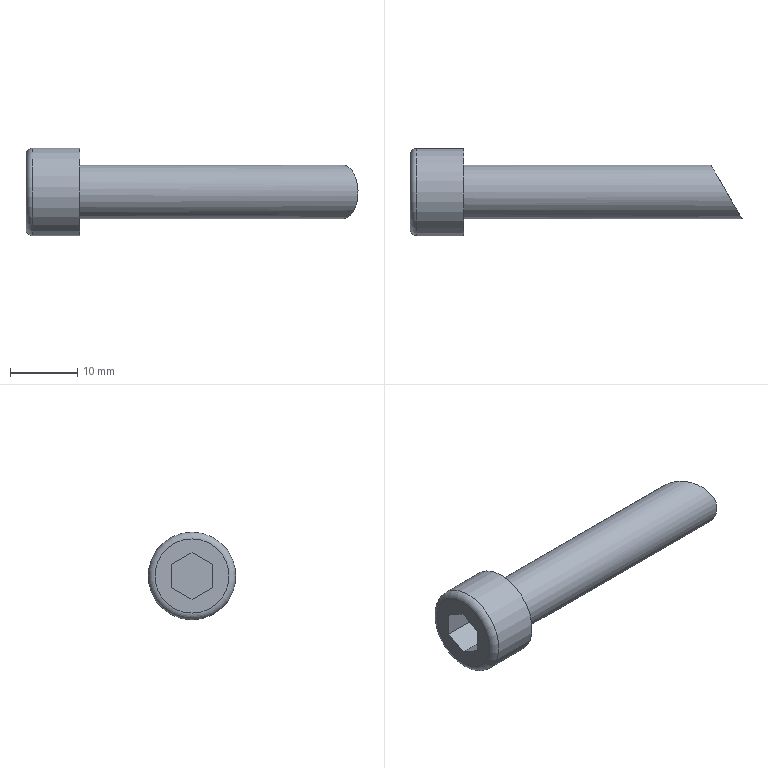Part | STEP file | Tube necking machine_id610_x_t | 1 solid | 13 faces | box 49.238 x 13 x 13 mm | volume 2846 mm3 | plane 10 | cylinder 2 | torus 1 | commonest cylinder face diameters 8 x1 13 x1
STEP:
#1=CARTESIAN_POINT('',(0.,0.,0.));
#2=DIRECTION('',(0.,0.,1.));
#3=DIRECTION('',(1.,0.,0.));
#4=AXIS2_PLACEMENT_3D('',#1,#2,#3);
#5=CARTESIAN_POINT('',(367.5,30.,164.5));
#6=VERTEX_POINT('',#5);
#7=CARTESIAN_POINT('',(367.5,30.,170.));
#8=DIRECTION('',(-1.,0.,0.));
#9=DIRECTION('',(0.,0.,-1.));
#10=AXIS2_PLACEMENT_3D('',#7,#8,#9);
#11=CIRCLE('',#10,5.5);
#12=CARTESIAN_POINT('',(367.5,30.,176.5));
#13=DIRECTION('',(1.,0.,0.));
#14=DIRECTION('',(0.,0.,-1.));
#15=AXIS2_PLACEMENT_3D('',#12,#13,#14);
#16=PLANE('',#15);
#17=CARTESIAN_POINT('',(12.,0.));
#18=CARTESIAN_POINT('',(12.,-9.526));
#19=CARTESIAN_POINT('',(3.75,-4.763));
#20=CARTESIAN_POINT('',(-4.5,0.));
#21=CARTESIAN_POINT('',(3.75,4.763));
#22=CARTESIAN_POINT('',(12.,9.526));
#23=CARTESIAN_POINT('',(12.,0.));
#24=(BOUNDED_CURVE()B_SPLINE_CURVE(2,(#17,#18,#19,#20,#21,#22,#23),.UNSPECIFIED.,.T.,.F.)B_SPLINE_CURVE_WITH_KNOTS((1,2,2,2,2,1),(-2.094,0.,2.094,4.189,6.283,8.378),.UNSPECIFIED.)CURVE()GEOMETRIC_REPRESENTATION_ITEM()RATIONAL_B_SPLINE_CURVE((1.,0.5,1.,0.5,1.,0.5,1.))REPRESENTATION_ITEM(''));
#25=(GEOMETRIC_REPRESENTATION_CONTEXT(2)PARAMETRIC_REPRESENTATION_CONTEXT()REPRESENTATION_CONTEXT('',''));
#26=DEFINITIONAL_REPRESENTATION('',(#24),#25);
#27=PCURVE('',#16,#26);
#28=CARTESIAN_POINT('',(368.5,30.,170.));
#29=DIRECTION('',(1.,0.,0.));
#30=DIRECTION('',(0.,0.,-1.));
#31=AXIS2_PLACEMENT_3D('',#28,#29,#30);
#32=TOROIDAL_SURFACE('',#31,5.5,1.);
#33=CARTESIAN_POINT('',(6.283,4.712));
#34=DIRECTION('',(-1.,0.));
#35=VECTOR('',#34,1.);
#36=LINE('',#33,#35);
#37=(GEOMETRIC_REPRESENTATION_CONTEXT(2)PARAMETRIC_REPRESENTATION_CONTEXT()REPRESENTATION_CONTEXT('',''));
#38=DEFINITIONAL_REPRESENTATION('',(#36),#37);
#39=PCURVE('',#32,#38);
#40=SURFACE_CURVE('',#11,(#27,#39),.PCURVE_S1.);
#41=EDGE_CURVE('',#6,#6,#40,.T.);
#42=ORIENTED_EDGE('',*,*,#41,.T.);
#43=EDGE_LOOP('',(#42));
#44=FACE_BOUND('',#43,.T.);
#45=CARTESIAN_POINT('',(367.5,33.,168.268));
#46=VERTEX_POINT('',#45);
#47=CARTESIAN_POINT('',(367.5,33.,171.732));
#48=VERTEX_POINT('',#47);
#49=CARTESIAN_POINT('',(367.5,33.,168.268));
#50=DIRECTION('',(0.,0.,1.));
#51=VECTOR('',#50,1.);
#52=LINE('',#49,#51);
#53=CARTESIAN_POINT('',(8.232,3.));
#54=DIRECTION('',(-1.,0.));
#55=VECTOR('',#54,1.);
#56=LINE('',#53,#55);
#57=(GEOMETRIC_REPRESENTATION_CONTEXT(2)PARAMETRIC_REPRESENTATION_CONTEXT()REPRESENTATION_CONTEXT('',''));
#58=DEFINITIONAL_REPRESENTATION('',(#56),#57);
#59=PCURVE('',#16,#58);
#60=CARTESIAN_POINT('',(372.78,33.,168.268));
#61=DIRECTION('',(0.,-1.,0.));
#62=DIRECTION('',(0.,0.,1.));
#63=AXIS2_PLACEMENT_3D('',#60,#61,#62);
#64=PLANE('',#63);
#65=CARTESIAN_POINT('',(0.,5.28));
#66=DIRECTION('',(1.,0.));
#67=VECTOR('',#66,1.);
#68=LINE('',#65,#67);
#69=(GEOMETRIC_REPRESENTATION_CONTEXT(2)PARAMETRIC_REPRESENTATION_CONTEXT()REPRESENTATION_CONTEXT('',''));
#70=DEFINITIONAL_REPRESENTATION('',(#68),#69);
#71=PCURVE('',#64,#70);
#72=SURFACE_CURVE('',#52,(#59,#71),.PCURVE_S1.);
#73=EDGE_CURVE('',#46,#48,#72,.T.);
#74=ORIENTED_EDGE('',*,*,#73,.T.);
#75=CARTESIAN_POINT('',(367.5,30.,173.464));
#76=VERTEX_POINT('',#75);
#77=CARTESIAN_POINT('',(367.5,33.,171.732));
#78=DIRECTION('',(0.,-0.866,0.5));
#79=VECTOR('',#78,1.);
#80=LINE('',#77,#79);
#81=CARTESIAN_POINT('',(4.768,3.));
#82=DIRECTION('',(-0.5,-0.866));
#83=VECTOR('',#82,1.);
#84=LINE('',#81,#83);
#85=(GEOMETRIC_REPRESENTATION_CONTEXT(2)PARAMETRIC_REPRESENTATION_CONTEXT()REPRESENTATION_CONTEXT('',''));
#86=DEFINITIONAL_REPRESENTATION('',(#84),#85);
#87=PCURVE('',#16,#86);
#88=CARTESIAN_POINT('',(372.78,33.,171.732));
#89=DIRECTION('',(0.,-0.5,-0.866));
#90=DIRECTION('',(0.,-0.866,0.5));
#91=AXIS2_PLACEMENT_3D('',#88,#89,#90);
#92=PLANE('',#91);
#93=CARTESIAN_POINT('',(0.,5.28));
#94=DIRECTION('',(1.,0.));
#95=VECTOR('',#94,1.);
#96=LINE('',#93,#95);
#97=(GEOMETRIC_REPRESENTATION_CONTEXT(2)PARAMETRIC_REPRESENTATION_CONTEXT()REPRESENTATION_CONTEXT('',''));
#98=DEFINITIONAL_REPRESENTATION('',(#96),#97);
#99=PCURVE('',#92,#98);
#100=SURFACE_CURVE('',#80,(#87,#99),.PCURVE_S1.);
#101=EDGE_CURVE('',#48,#76,#100,.T.);
#102=ORIENTED_EDGE('',*,*,#101,.T.);
#103=CARTESIAN_POINT('',(367.5,27.,171.732));
#104=VERTEX_POINT('',#103);
#105=CARTESIAN_POINT('',(367.5,30.,173.464));
#106=DIRECTION('',(0.,-0.866,-0.5));
#107=VECTOR('',#106,1.);
#108=LINE('',#105,#107);
#109=CARTESIAN_POINT('',(3.036,0.));
#110=DIRECTION('',(0.5,-0.866));
#111=VECTOR('',#110,1.);
#112=LINE('',#109,#111);
#113=(GEOMETRIC_REPRESENTATION_CONTEXT(2)PARAMETRIC_REPRESENTATION_CONTEXT()REPRESENTATION_CONTEXT('',''));
#114=DEFINITIONAL_REPRESENTATION('',(#112),#113);
#115=PCURVE('',#16,#114);
#116=CARTESIAN_POINT('',(372.78,30.,173.464));
#117=DIRECTION('',(0.,0.5,-0.866));
#118=DIRECTION('',(0.,-0.866,-0.5));
#119=AXIS2_PLACEMENT_3D('',#116,#117,#118);
#120=PLANE('',#119);
#121=CARTESIAN_POINT('',(0.,5.28));
#122=DIRECTION('',(1.,0.));
#123=VECTOR('',#122,1.);
#124=LINE('',#121,#123);
#125=(GEOMETRIC_REPRESENTATION_CONTEXT(2)PARAMETRIC_REPRESENTATION_CONTEXT()REPRESENTATION_CONTEXT('',''));
#126=DEFINITIONAL_REPRESENTATION('',(#124),#125);
#127=PCURVE('',#120,#126);
#128=SURFACE_CURVE('',#108,(#115,#127),.PCURVE_S1.);
#129=EDGE_CURVE('',#76,#104,#128,.T.);
#130=ORIENTED_EDGE('',*,*,#129,.T.);
#131=CARTESIAN_POINT('',(367.5,27.,168.268));
#132=VERTEX_POINT('',#131);
#133=CARTESIAN_POINT('',(367.5,27.,171.732));
#134=DIRECTION('',(0.,0.,-1.));
#135=VECTOR('',#134,1.);
#136=LINE('',#133,#135);
#137=CARTESIAN_POINT('',(4.768,-3.));
#138=DIRECTION('',(1.,0.));
#139=VECTOR('',#138,1.);
#140=LINE('',#137,#139);
#141=(GEOMETRIC_REPRESENTATION_CONTEXT(2)PARAMETRIC_REPRESENTATION_CONTEXT()REPRESENTATION_CONTEXT('',''));
#142=DEFINITIONAL_REPRESENTATION('',(#140),#141);
#143=PCURVE('',#16,#142);
#144=CARTESIAN_POINT('',(372.78,27.,171.732));
#145=DIRECTION('',(0.,1.,0.));
#146=DIRECTION('',(0.,0.,-1.));
#147=AXIS2_PLACEMENT_3D('',#144,#145,#146);
#148=PLANE('',#147);
#149=CARTESIAN_POINT('',(0.,5.28));
#150=DIRECTION('',(1.,0.));
#151=VECTOR('',#150,1.);
#152=LINE('',#149,#151);
#153=(GEOMETRIC_REPRESENTATION_CONTEXT(2)PARAMETRIC_REPRESENTATION_CONTEXT()REPRESENTATION_CONTEXT('',''));
#154=DEFINITIONAL_REPRESENTATION('',(#152),#153);
#155=PCURVE('',#148,#154);
#156=SURFACE_CURVE('',#136,(#143,#155),.PCURVE_S1.);
#157=EDGE_CURVE('',#104,#132,#156,.T.);
#158=ORIENTED_EDGE('',*,*,#157,.T.);
#159=CARTESIAN_POINT('',(367.5,30.,166.536));
#160=VERTEX_POINT('',#159);
#161=CARTESIAN_POINT('',(367.5,27.,168.268));
#162=DIRECTION('',(0.,0.866,-0.5));
#163=VECTOR('',#162,1.);
#164=LINE('',#161,#163);
#165=CARTESIAN_POINT('',(8.232,-3.));
#166=DIRECTION('',(0.5,0.866));
#167=VECTOR('',#166,1.);
#168=LINE('',#165,#167);
#169=(GEOMETRIC_REPRESENTATION_CONTEXT(2)PARAMETRIC_REPRESENTATION_CONTEXT()REPRESENTATION_CONTEXT('',''));
#170=DEFINITIONAL_REPRESENTATION('',(#168),#169);
#171=PCURVE('',#16,#170);
#172=CARTESIAN_POINT('',(372.78,27.,168.268));
#173=DIRECTION('',(0.,0.5,0.866));
#174=DIRECTION('',(0.,0.866,-0.5));
#175=AXIS2_PLACEMENT_3D('',#172,#173,#174);
#176=PLANE('',#175);
#177=CARTESIAN_POINT('',(0.,5.28));
#178=DIRECTION('',(1.,0.));
#179=VECTOR('',#178,1.);
#180=LINE('',#177,#179);
#181=(GEOMETRIC_REPRESENTATION_CONTEXT(2)PARAMETRIC_REPRESENTATION_CONTEXT()REPRESENTATION_CONTEXT('',''));
#182=DEFINITIONAL_REPRESENTATION('',(#180),#181);
#183=PCURVE('',#176,#182);
#184=SURFACE_CURVE('',#164,(#171,#183),.PCURVE_S1.);
#185=EDGE_CURVE('',#132,#160,#184,.T.);
#186=ORIENTED_EDGE('',*,*,#185,.T.);
#187=CARTESIAN_POINT('',(367.5,30.,166.536));
#188=DIRECTION('',(0.,0.866,0.5));
#189=VECTOR('',#188,1.);
#190=LINE('',#187,#189);
#191=CARTESIAN_POINT('',(9.964,0.));
#192=DIRECTION('',(-0.5,0.866));
#193=VECTOR('',#192,1.);
#194=LINE('',#191,#193);
#195=(GEOMETRIC_REPRESENTATION_CONTEXT(2)PARAMETRIC_REPRESENTATION_CONTEXT()REPRESENTATION_CONTEXT('',''));
#196=DEFINITIONAL_REPRESENTATION('',(#194),#195);
#197=PCURVE('',#16,#196);
#198=CARTESIAN_POINT('',(372.78,30.,166.536));
#199=DIRECTION('',(0.,-0.5,0.866));
#200=DIRECTION('',(0.,0.866,0.5));
#201=AXIS2_PLACEMENT_3D('',#198,#199,#200);
#202=PLANE('',#201);
#203=CARTESIAN_POINT('',(0.,5.28));
#204=DIRECTION('',(1.,0.));
#205=VECTOR('',#204,1.);
#206=LINE('',#203,#205);
#207=(GEOMETRIC_REPRESENTATION_CONTEXT(2)PARAMETRIC_REPRESENTATION_CONTEXT()REPRESENTATION_CONTEXT('',''));
#208=DEFINITIONAL_REPRESENTATION('',(#206),#207);
#209=PCURVE('',#202,#208);
#210=SURFACE_CURVE('',#190,(#197,#209),.PCURVE_S1.);
#211=EDGE_CURVE('',#160,#46,#210,.T.);
#212=ORIENTED_EDGE('',*,*,#211,.T.);
#213=EDGE_LOOP('',(#74,#102,#130,#158,#186,#212));
#214=FACE_BOUND('',#213,.T.);
#215=ADVANCED_FACE('',(#44,#214),#16,.F.);
#216=CARTESIAN_POINT('',(368.5,30.,163.5));
#217=VERTEX_POINT('',#216);
#218=CARTESIAN_POINT('',(368.5,30.,176.5));
#219=VERTEX_POINT('',#218);
#220=CARTESIAN_POINT('',(368.5,30.,170.));
#221=DIRECTION('',(1.,0.,0.));
#222=DIRECTION('',(0.,0.,-1.));
#223=AXIS2_PLACEMENT_3D('',#220,#221,#222);
#224=CIRCLE('',#223,6.5);
#225=CARTESIAN_POINT('',(374.4,30.,170.));
#226=DIRECTION('',(-1.,0.,0.));
#227=DIRECTION('',(0.,0.,1.));
#228=AXIS2_PLACEMENT_3D('',#225,#226,#227);
#229=CYLINDRICAL_SURFACE('',#228,6.5);
#230=CARTESIAN_POINT('',(3.142,5.9));
#231=DIRECTION('',(-1.,0.));
#232=VECTOR('',#231,1.);
#233=LINE('',#230,#232);
#234=(GEOMETRIC_REPRESENTATION_CONTEXT(2)PARAMETRIC_REPRESENTATION_CONTEXT()REPRESENTATION_CONTEXT('',''));
#235=DEFINITIONAL_REPRESENTATION('',(#233),#234);
#236=PCURVE('',#229,#235);
#237=CARTESIAN_POINT('',(0.,6.283));
#238=DIRECTION('',(1.,0.));
#239=VECTOR('',#238,1.);
#240=LINE('',#237,#239);
#241=(GEOMETRIC_REPRESENTATION_CONTEXT(2)PARAMETRIC_REPRESENTATION_CONTEXT()REPRESENTATION_CONTEXT('',''));
#242=DEFINITIONAL_REPRESENTATION('',(#240),#241);
#243=PCURVE('',#32,#242);
#244=SURFACE_CURVE('',#224,(#236,#243),.PCURVE_S1.);
#245=EDGE_CURVE('',#217,#219,#244,.T.);
#246=ORIENTED_EDGE('',*,*,#245,.T.);
#247=CARTESIAN_POINT('',(375.5,30.,176.5));
#248=VERTEX_POINT('',#247);
#249=CARTESIAN_POINT('',(375.5,30.,176.5));
#250=CARTESIAN_POINT('',(368.5,30.,176.5));
#251=B_SPLINE_CURVE_WITH_KNOTS('',1,(#249,#250),.UNSPECIFIED.,.F.,.F.,(2,2),(-1.1,5.9),.PIECEWISE_BEZIER_KNOTS.);
#252=CARTESIAN_POINT('',(0.,0.));
#253=DIRECTION('',(0.,1.));
#254=VECTOR('',#253,1.);
#255=LINE('',#252,#254);
#256=(GEOMETRIC_REPRESENTATION_CONTEXT(2)PARAMETRIC_REPRESENTATION_CONTEXT()REPRESENTATION_CONTEXT('',''));
#257=DEFINITIONAL_REPRESENTATION('',(#255),#256);
#258=PCURVE('',#229,#257);
#259=CARTESIAN_POINT('',(6.283,0.));
#260=DIRECTION('',(0.,1.));
#261=VECTOR('',#260,1.);
#262=LINE('',#259,#261);
#263=(GEOMETRIC_REPRESENTATION_CONTEXT(2)PARAMETRIC_REPRESENTATION_CONTEXT()REPRESENTATION_CONTEXT('',''));
#264=DEFINITIONAL_REPRESENTATION('',(#262),#263);
#265=PCURVE('',#229,#264);
#266=SEAM_CURVE('',#251,(#258,#265),.PCURVE_S1.);
#267=EDGE_CURVE('',#248,#219,#266,.T.);
#268=ORIENTED_EDGE('',*,*,#267,.F.);
#269=CARTESIAN_POINT('',(375.5,30.,170.));
#270=DIRECTION('',(-1.,0.,0.));
#271=DIRECTION('',(0.,0.,1.));
#272=AXIS2_PLACEMENT_3D('',#269,#270,#271);
#273=CIRCLE('',#272,6.5);
#274=CARTESIAN_POINT('',(0.,-1.1));
#275=DIRECTION('',(1.,0.));
#276=VECTOR('',#275,1.);
#277=LINE('',#274,#276);
#278=(GEOMETRIC_REPRESENTATION_CONTEXT(2)PARAMETRIC_REPRESENTATION_CONTEXT()REPRESENTATION_CONTEXT('',''));
#279=DEFINITIONAL_REPRESENTATION('',(#277),#278);
#280=PCURVE('',#229,#279);
#281=CARTESIAN_POINT('',(375.5,30.,174.));
#282=DIRECTION('',(-1.,0.,0.));
#283=DIRECTION('',(0.,0.,1.));
#284=AXIS2_PLACEMENT_3D('',#281,#282,#283);
#285=PLANE('',#284);
#286=CARTESIAN_POINT('',(-4.,0.));
#287=DIRECTION('',(1.,0.));
#288=AXIS2_PLACEMENT_2D('',#286,#287);
#289=CIRCLE('',#288,6.5);
#290=(GEOMETRIC_REPRESENTATION_CONTEXT(2)PARAMETRIC_REPRESENTATION_CONTEXT()REPRESENTATION_CONTEXT('',''));
#291=DEFINITIONAL_REPRESENTATION('',(#289),#290);
#292=PCURVE('',#285,#291);
#293=SURFACE_CURVE('',#273,(#280,#292),.PCURVE_S1.);
#294=EDGE_CURVE('',#248,#248,#293,.T.);
#295=ORIENTED_EDGE('',*,*,#294,.T.);
#296=ORIENTED_EDGE('',*,*,#267,.T.);
#297=CARTESIAN_POINT('',(368.5,30.,170.));
#298=DIRECTION('',(1.,0.,0.));
#299=DIRECTION('',(0.,0.,-1.));
#300=AXIS2_PLACEMENT_3D('',#297,#298,#299);
#301=CIRCLE('',#300,6.5);
#302=CARTESIAN_POINT('',(9.425,5.9));
#303=DIRECTION('',(-1.,0.));
#304=VECTOR('',#303,1.);
#305=LINE('',#302,#304);
#306=(GEOMETRIC_REPRESENTATION_CONTEXT(2)PARAMETRIC_REPRESENTATION_CONTEXT()REPRESENTATION_CONTEXT('',''));
#307=DEFINITIONAL_REPRESENTATION('',(#305),#306);
#308=PCURVE('',#229,#307);
#309=CARTESIAN_POINT('',(0.,6.283));
#310=DIRECTION('',(1.,0.));
#311=VECTOR('',#310,1.);
#312=LINE('',#309,#311);
#313=(GEOMETRIC_REPRESENTATION_CONTEXT(2)PARAMETRIC_REPRESENTATION_CONTEXT()REPRESENTATION_CONTEXT('',''));
#314=DEFINITIONAL_REPRESENTATION('',(#312),#313);
#315=PCURVE('',#32,#314);
#316=SURFACE_CURVE('',#301,(#308,#315),.PCURVE_S1.);
#317=EDGE_CURVE('',#219,#217,#316,.T.);
#318=ORIENTED_EDGE('',*,*,#317,.T.);
#319=EDGE_LOOP('',(#246,#268,#295,#296,#318));
#320=FACE_BOUND('',#319,.T.);
#321=ADVANCED_FACE('',(#320),#229,.T.);
#322=ORIENTED_EDGE('',*,*,#294,.F.);
#323=EDGE_LOOP('',(#322));
#324=FACE_BOUND('',#323,.T.);
#325=CARTESIAN_POINT('',(375.5,30.,174.));
#326=VERTEX_POINT('',#325);
#327=CARTESIAN_POINT('',(375.5,30.,170.));
#328=DIRECTION('',(-1.,0.,0.));
#329=DIRECTION('',(0.,0.,1.));
#330=AXIS2_PLACEMENT_3D('',#327,#328,#329);
#331=CIRCLE('',#330,4.);
#332=CARTESIAN_POINT('',(-4.,0.));
#333=DIRECTION('',(1.,0.));
#334=AXIS2_PLACEMENT_2D('',#332,#333);
#335=CIRCLE('',#334,4.);
#336=(GEOMETRIC_REPRESENTATION_CONTEXT(2)PARAMETRIC_REPRESENTATION_CONTEXT()REPRESENTATION_CONTEXT('',''));
#337=DEFINITIONAL_REPRESENTATION('',(#335),#336);
#338=PCURVE('',#285,#337);
#339=CARTESIAN_POINT('',(374.4,30.,170.));
#340=DIRECTION('',(-1.,0.,0.));
#341=DIRECTION('',(0.,0.,1.));
#342=AXIS2_PLACEMENT_3D('',#339,#340,#341);
#343=CYLINDRICAL_SURFACE('',#342,4.);
#344=CARTESIAN_POINT('',(0.,-1.1));
#345=DIRECTION('',(1.,0.));
#346=VECTOR('',#345,1.);
#347=LINE('',#344,#346);
#348=(GEOMETRIC_REPRESENTATION_CONTEXT(2)PARAMETRIC_REPRESENTATION_CONTEXT()REPRESENTATION_CONTEXT('',''));
#349=DEFINITIONAL_REPRESENTATION('',(#347),#348);
#350=PCURVE('',#343,#349);
#351=SURFACE_CURVE('',#331,(#338,#350),.PCURVE_S1.);
#352=EDGE_CURVE('',#326,#326,#351,.T.);
#353=ORIENTED_EDGE('',*,*,#352,.T.);
#354=EDGE_LOOP('',(#353));
#355=FACE_BOUND('',#354,.T.);
#356=ADVANCED_FACE('',(#324,#355),#285,.F.);
#357=ORIENTED_EDGE('',*,*,#352,.F.);
#358=CARTESIAN_POINT('',(414.428,30.,174.));
#359=VERTEX_POINT('',#358);
#360=CARTESIAN_POINT('',(414.428,30.,174.));
#361=CARTESIAN_POINT('',(375.5,30.,174.));
#362=B_SPLINE_CURVE_WITH_KNOTS('',1,(#360,#361),.UNSPECIFIED.,.F.,.F.,(2,2),(-40.028,-1.1),.PIECEWISE_BEZIER_KNOTS.);
#363=CARTESIAN_POINT('',(0.,0.));
#364=DIRECTION('',(0.,1.));
#365=VECTOR('',#364,1.);
#366=LINE('',#363,#365);
#367=(GEOMETRIC_REPRESENTATION_CONTEXT(2)PARAMETRIC_REPRESENTATION_CONTEXT()REPRESENTATION_CONTEXT('',''));
#368=DEFINITIONAL_REPRESENTATION('',(#366),#367);
#369=PCURVE('',#343,#368);
#370=CARTESIAN_POINT('',(6.283,0.));
#371=DIRECTION('',(0.,1.));
#372=VECTOR('',#371,1.);
#373=LINE('',#370,#372);
#374=(GEOMETRIC_REPRESENTATION_CONTEXT(2)PARAMETRIC_REPRESENTATION_CONTEXT()REPRESENTATION_CONTEXT('',''));
#375=DEFINITIONAL_REPRESENTATION('',(#373),#374);
#376=PCURVE('',#343,#375);
#377=SEAM_CURVE('',#362,(#369,#376),.PCURVE_S1.);
#378=EDGE_CURVE('',#359,#326,#377,.T.);
#379=ORIENTED_EDGE('',*,*,#378,.F.);
#380=CARTESIAN_POINT('',(412.119,34.,170.));
#381=VERTEX_POINT('',#380);
#382=CARTESIAN_POINT('',(414.428,30.,170.));
#383=DIRECTION('',(-0.866,-0.5,0.));
#384=DIRECTION('',(-0.5,0.866,0.));
#385=AXIS2_PLACEMENT_3D('',#382,#383,#384);
#386=ELLIPSE('',#385,4.619,4.);
#387=CARTESIAN_POINT('',(-4.712,-37.719));
#388=CARTESIAN_POINT('',(-4.617,-37.718));
#389=CARTESIAN_POINT('',(-4.427,-37.783));
#390=CARTESIAN_POINT('',(-4.141,-38.059));
#391=CARTESIAN_POINT('',(-3.856,-38.495));
#392=CARTESIAN_POINT('',(-3.57,-39.056));
#393=CARTESIAN_POINT('',(-3.284,-39.695));
#394=CARTESIAN_POINT('',(-2.999,-40.361));
#395=CARTESIAN_POINT('',(-2.713,-41.001));
#396=CARTESIAN_POINT('',(-2.428,-41.561));
#397=CARTESIAN_POINT('',(-2.142,-41.998));
#398=CARTESIAN_POINT('',(-1.856,-42.274));
#399=CARTESIAN_POINT('',(-1.571,-42.369));
#400=CARTESIAN_POINT('',(-1.285,-42.274));
#401=CARTESIAN_POINT('',(-0.9996,-41.998));
#402=CARTESIAN_POINT('',(-0.714,-41.561));
#403=CARTESIAN_POINT('',(-0.4284,-41.001));
#404=CARTESIAN_POINT('',(-0.1428,-40.361));
#405=CARTESIAN_POINT('',(0.1428,-39.695));
#406=CARTESIAN_POINT('',(0.4284,-39.056));
#407=CARTESIAN_POINT('',(0.714,-38.495));
#408=CARTESIAN_POINT('',(0.9996,-38.059));
#409=CARTESIAN_POINT('',(1.285,-37.783));
#410=CARTESIAN_POINT('',(1.476,-37.718));
#411=CARTESIAN_POINT('',(1.571,-37.719));
#412=B_SPLINE_CURVE_WITH_KNOTS('',3,(#387,#388,#389,#390,#391,#392,#393,#394,#395,#396,#397,#398,#399,#400,#401,#402,#403,#404,#405,#406,#407,#408,#409,#410,#411),.UNSPECIFIED.,.F.,.F.,(4,1,1,1,1,1,1,1,1,1,1,1,1,1,1,1,1,1,1,1,1,1,4),(0.,0.2856,0.5712,0.8568,1.142,1.428,1.714,1.999,2.285,2.57,2.856,3.142,3.427,3.713,3.998,4.284,4.57,4.855,5.141,5.426,5.712,5.998,6.283),.QUASI_UNIFORM_KNOTS.);
#413=(GEOMETRIC_REPRESENTATION_CONTEXT(2)PARAMETRIC_REPRESENTATION_CONTEXT()REPRESENTATION_CONTEXT('',''));
#414=DEFINITIONAL_REPRESENTATION('',(#412),#413);
#415=PCURVE('',#343,#414);
#416=CARTESIAN_POINT('',(414.036,30.679,170.));
#417=DIRECTION('',(-0.866,-0.5,0.));
#418=DIRECTION('',(0.,0.,1.));
#419=AXIS2_PLACEMENT_3D('',#416,#417,#418);
#420=PLANE('',#419);
#421=CARTESIAN_POINT('',(0.,-0.7846));
#422=DIRECTION('',(0.,1.));
#423=AXIS2_PLACEMENT_2D('',#421,#422);
#424=ELLIPSE('',#423,4.619,4.);
#425=(GEOMETRIC_REPRESENTATION_CONTEXT(2)PARAMETRIC_REPRESENTATION_CONTEXT()REPRESENTATION_CONTEXT('',''));
#426=DEFINITIONAL_REPRESENTATION('',(#424),#425);
#427=PCURVE('',#420,#426);
#428=SURFACE_CURVE('',#386,(#415,#427),.PCURVE_S1.);
#429=EDGE_CURVE('',#359,#381,#428,.T.);
#430=ORIENTED_EDGE('',*,*,#429,.T.);
#431=CARTESIAN_POINT('',(414.428,30.,170.));
#432=DIRECTION('',(-0.866,-0.5,0.));
#433=DIRECTION('',(-0.5,0.866,0.));
#434=AXIS2_PLACEMENT_3D('',#431,#432,#433);
#435=ELLIPSE('',#434,4.619,4.);
#436=CARTESIAN_POINT('',(1.571,-37.719));
#437=CARTESIAN_POINT('',(1.666,-37.718));
#438=CARTESIAN_POINT('',(1.856,-37.783));
#439=CARTESIAN_POINT('',(2.142,-38.059));
#440=CARTESIAN_POINT('',(2.428,-38.495));
#441=CARTESIAN_POINT('',(2.713,-39.056));
#442=CARTESIAN_POINT('',(2.999,-39.695));
#443=CARTESIAN_POINT('',(3.284,-40.361));
#444=CARTESIAN_POINT('',(3.57,-41.001));
#445=CARTESIAN_POINT('',(3.856,-41.561));
#446=CARTESIAN_POINT('',(4.141,-41.998));
#447=CARTESIAN_POINT('',(4.427,-42.274));
#448=CARTESIAN_POINT('',(4.712,-42.369));
#449=CARTESIAN_POINT('',(4.998,-42.274));
#450=CARTESIAN_POINT('',(5.284,-41.998));
#451=CARTESIAN_POINT('',(5.569,-41.561));
#452=CARTESIAN_POINT('',(5.855,-41.001));
#453=CARTESIAN_POINT('',(6.14,-40.361));
#454=CARTESIAN_POINT('',(6.426,-39.695));
#455=CARTESIAN_POINT('',(6.712,-39.056));
#456=CARTESIAN_POINT('',(6.997,-38.495));
#457=CARTESIAN_POINT('',(7.283,-38.059));
#458=CARTESIAN_POINT('',(7.568,-37.783));
#459=CARTESIAN_POINT('',(7.759,-37.718));
#460=CARTESIAN_POINT('',(7.854,-37.719));
#461=B_SPLINE_CURVE_WITH_KNOTS('',3,(#436,#437,#438,#439,#440,#441,#442,#443,#444,#445,#446,#447,#448,#449,#450,#451,#452,#453,#454,#455,#456,#457,#458,#459,#460),.UNSPECIFIED.,.F.,.F.,(4,1,1,1,1,1,1,1,1,1,1,1,1,1,1,1,1,1,1,1,1,1,4),(0.,0.2856,0.5712,0.8568,1.142,1.428,1.714,1.999,2.285,2.57,2.856,3.142,3.427,3.713,3.998,4.284,4.57,4.855,5.141,5.426,5.712,5.998,6.283),.QUASI_UNIFORM_KNOTS.);
#462=(GEOMETRIC_REPRESENTATION_CONTEXT(2)PARAMETRIC_REPRESENTATION_CONTEXT()REPRESENTATION_CONTEXT('',''));
#463=DEFINITIONAL_REPRESENTATION('',(#461),#462);
#464=PCURVE('',#343,#463);
#465=CARTESIAN_POINT('',(0.,-0.7846));
#466=DIRECTION('',(0.,1.));
#467=AXIS2_PLACEMENT_2D('',#465,#466);
#468=ELLIPSE('',#467,4.619,4.);
#469=(GEOMETRIC_REPRESENTATION_CONTEXT(2)PARAMETRIC_REPRESENTATION_CONTEXT()REPRESENTATION_CONTEXT('',''));
#470=DEFINITIONAL_REPRESENTATION('',(#468),#469);
#471=PCURVE('',#420,#470);
#472=SURFACE_CURVE('',#435,(#464,#471),.PCURVE_S1.);
#473=EDGE_CURVE('',#381,#359,#472,.T.);
#474=ORIENTED_EDGE('',*,*,#473,.T.);
#475=ORIENTED_EDGE('',*,*,#378,.T.);
#476=EDGE_LOOP('',(#357,#379,#430,#474,#475));
#477=FACE_BOUND('',#476,.T.);
#478=ADVANCED_FACE('',(#477),#343,.T.);
#479=ORIENTED_EDGE('',*,*,#473,.F.);
#480=ORIENTED_EDGE('',*,*,#429,.F.);
#481=EDGE_LOOP('',(#479,#480));
#482=FACE_BOUND('',#481,.T.);
#483=ADVANCED_FACE('',(#482),#420,.F.);
#484=ORIENTED_EDGE('',*,*,#73,.F.);
#485=CARTESIAN_POINT('',(372.78,33.,168.268));
#486=VERTEX_POINT('',#485);
#487=CARTESIAN_POINT('',(372.78,33.,168.268));
#488=DIRECTION('',(1.,0.,0.));
#489=VECTOR('',#488,1.);
#490=LINE('',#487,#489);
#491=CARTESIAN_POINT('',(0.,0.));
#492=DIRECTION('',(0.,-1.));
#493=VECTOR('',#492,1.);
#494=LINE('',#491,#493);
#495=(GEOMETRIC_REPRESENTATION_CONTEXT(2)PARAMETRIC_REPRESENTATION_CONTEXT()REPRESENTATION_CONTEXT('',''));
#496=DEFINITIONAL_REPRESENTATION('',(#494),#495);
#497=PCURVE('',#64,#496);
#498=CARTESIAN_POINT('',(3.464,0.));
#499=DIRECTION('',(0.,-1.));
#500=VECTOR('',#499,1.);
#501=LINE('',#498,#500);
#502=(GEOMETRIC_REPRESENTATION_CONTEXT(2)PARAMETRIC_REPRESENTATION_CONTEXT()REPRESENTATION_CONTEXT('',''));
#503=DEFINITIONAL_REPRESENTATION('',(#501),#502);
#504=PCURVE('',#202,#503);
#505=SURFACE_CURVE('',#490,(#497,#504),.PCURVE_S1.);
#506=EDGE_CURVE('',#46,#486,#505,.T.);
#507=ORIENTED_EDGE('',*,*,#506,.T.);
#508=CARTESIAN_POINT('',(372.78,33.,171.732));
#509=VERTEX_POINT('',#508);
#510=CARTESIAN_POINT('',(372.78,33.,168.268));
#511=DIRECTION('',(0.,0.,-1.));
#512=VECTOR('',#511,1.);
#513=LINE('',#510,#512);
#514=CARTESIAN_POINT('',(0.,0.));
#515=DIRECTION('',(-1.,0.));
#516=VECTOR('',#515,1.);
#517=LINE('',#514,#516);
#518=(GEOMETRIC_REPRESENTATION_CONTEXT(2)PARAMETRIC_REPRESENTATION_CONTEXT()REPRESENTATION_CONTEXT('',''));
#519=DEFINITIONAL_REPRESENTATION('',(#517),#518);
#520=PCURVE('',#64,#519);
#521=CARTESIAN_POINT('',(372.78,30.,170.));
#522=DIRECTION('',(1.,0.,0.));
#523=DIRECTION('',(0.,0.,-1.));
#524=AXIS2_PLACEMENT_3D('',#521,#522,#523);
#525=PLANE('',#524);
#526=CARTESIAN_POINT('',(1.732,3.));
#527=DIRECTION('',(1.,0.));
#528=VECTOR('',#527,1.);
#529=LINE('',#526,#528);
#530=(GEOMETRIC_REPRESENTATION_CONTEXT(2)PARAMETRIC_REPRESENTATION_CONTEXT()REPRESENTATION_CONTEXT('',''));
#531=DEFINITIONAL_REPRESENTATION('',(#529),#530);
#532=PCURVE('',#525,#531);
#533=SURFACE_CURVE('',#513,(#520,#532),.PCURVE_S1.);
#534=EDGE_CURVE('',#509,#486,#533,.T.);
#535=ORIENTED_EDGE('',*,*,#534,.F.);
#536=CARTESIAN_POINT('',(372.78,33.,171.732));
#537=DIRECTION('',(1.,0.,0.));
#538=VECTOR('',#537,1.);
#539=LINE('',#536,#538);
#540=CARTESIAN_POINT('',(3.464,0.));
#541=DIRECTION('',(0.,-1.));
#542=VECTOR('',#541,1.);
#543=LINE('',#540,#542);
#544=(GEOMETRIC_REPRESENTATION_CONTEXT(2)PARAMETRIC_REPRESENTATION_CONTEXT()REPRESENTATION_CONTEXT('',''));
#545=DEFINITIONAL_REPRESENTATION('',(#543),#544);
#546=PCURVE('',#64,#545);
#547=CARTESIAN_POINT('',(0.,0.));
#548=DIRECTION('',(0.,-1.));
#549=VECTOR('',#548,1.);
#550=LINE('',#547,#549);
#551=(GEOMETRIC_REPRESENTATION_CONTEXT(2)PARAMETRIC_REPRESENTATION_CONTEXT()REPRESENTATION_CONTEXT('',''));
#552=DEFINITIONAL_REPRESENTATION('',(#550),#551);
#553=PCURVE('',#92,#552);
#554=SURFACE_CURVE('',#539,(#546,#553),.PCURVE_S1.);
#555=EDGE_CURVE('',#48,#509,#554,.T.);
#556=ORIENTED_EDGE('',*,*,#555,.F.);
#557=EDGE_LOOP('',(#484,#507,#535,#556));
#558=FACE_BOUND('',#557,.T.);
#559=ADVANCED_FACE('',(#558),#64,.T.);
#560=ORIENTED_EDGE('',*,*,#101,.F.);
#561=ORIENTED_EDGE('',*,*,#555,.T.);
#562=CARTESIAN_POINT('',(372.78,30.,173.464));
#563=VERTEX_POINT('',#562);
#564=CARTESIAN_POINT('',(372.78,33.,171.732));
#565=DIRECTION('',(0.,0.866,-0.5));
#566=VECTOR('',#565,1.);
#567=LINE('',#564,#566);
#568=CARTESIAN_POINT('',(0.,0.));
#569=DIRECTION('',(-1.,0.));
#570=VECTOR('',#569,1.);
#571=LINE('',#568,#570);
#572=(GEOMETRIC_REPRESENTATION_CONTEXT(2)PARAMETRIC_REPRESENTATION_CONTEXT()REPRESENTATION_CONTEXT('',''));
#573=DEFINITIONAL_REPRESENTATION('',(#571),#572);
#574=PCURVE('',#92,#573);
#575=CARTESIAN_POINT('',(-1.732,3.));
#576=DIRECTION('',(0.5,0.866));
#577=VECTOR('',#576,1.);
#578=LINE('',#575,#577);
#579=(GEOMETRIC_REPRESENTATION_CONTEXT(2)PARAMETRIC_REPRESENTATION_CONTEXT()REPRESENTATION_CONTEXT('',''));
#580=DEFINITIONAL_REPRESENTATION('',(#578),#579);
#581=PCURVE('',#525,#580);
#582=SURFACE_CURVE('',#567,(#574,#581),.PCURVE_S1.);
#583=EDGE_CURVE('',#563,#509,#582,.T.);
#584=ORIENTED_EDGE('',*,*,#583,.F.);
#585=CARTESIAN_POINT('',(372.78,30.,173.464));
#586=DIRECTION('',(1.,0.,0.));
#587=VECTOR('',#586,1.);
#588=LINE('',#585,#587);
#589=CARTESIAN_POINT('',(3.464,0.));
#590=DIRECTION('',(0.,-1.));
#591=VECTOR('',#590,1.);
#592=LINE('',#589,#591);
#593=(GEOMETRIC_REPRESENTATION_CONTEXT(2)PARAMETRIC_REPRESENTATION_CONTEXT()REPRESENTATION_CONTEXT('',''));
#594=DEFINITIONAL_REPRESENTATION('',(#592),#593);
#595=PCURVE('',#92,#594);
#596=CARTESIAN_POINT('',(0.,0.));
#597=DIRECTION('',(0.,-1.));
#598=VECTOR('',#597,1.);
#599=LINE('',#596,#598);
#600=(GEOMETRIC_REPRESENTATION_CONTEXT(2)PARAMETRIC_REPRESENTATION_CONTEXT()REPRESENTATION_CONTEXT('',''));
#601=DEFINITIONAL_REPRESENTATION('',(#599),#600);
#602=PCURVE('',#120,#601);
#603=SURFACE_CURVE('',#588,(#595,#602),.PCURVE_S1.);
#604=EDGE_CURVE('',#76,#563,#603,.T.);
#605=ORIENTED_EDGE('',*,*,#604,.F.);
#606=EDGE_LOOP('',(#560,#561,#584,#605));
#607=FACE_BOUND('',#606,.T.);
#608=ADVANCED_FACE('',(#607),#92,.T.);
#609=ORIENTED_EDGE('',*,*,#129,.F.);
#610=ORIENTED_EDGE('',*,*,#604,.T.);
#611=CARTESIAN_POINT('',(372.78,27.,171.732));
#612=VERTEX_POINT('',#611);
#613=CARTESIAN_POINT('',(372.78,30.,173.464));
#614=DIRECTION('',(0.,0.866,0.5));
#615=VECTOR('',#614,1.);
#616=LINE('',#613,#615);
#617=CARTESIAN_POINT('',(0.,0.));
#618=DIRECTION('',(-1.,0.));
#619=VECTOR('',#618,1.);
#620=LINE('',#617,#619);
#621=(GEOMETRIC_REPRESENTATION_CONTEXT(2)PARAMETRIC_REPRESENTATION_CONTEXT()REPRESENTATION_CONTEXT('',''));
#622=DEFINITIONAL_REPRESENTATION('',(#620),#621);
#623=PCURVE('',#120,#622);
#624=CARTESIAN_POINT('',(-3.464,0.));
#625=DIRECTION('',(-0.5,0.866));
#626=VECTOR('',#625,1.);
#627=LINE('',#624,#626);
#628=(GEOMETRIC_REPRESENTATION_CONTEXT(2)PARAMETRIC_REPRESENTATION_CONTEXT()REPRESENTATION_CONTEXT('',''));
#629=DEFINITIONAL_REPRESENTATION('',(#627),#628);
#630=PCURVE('',#525,#629);
#631=SURFACE_CURVE('',#616,(#623,#630),.PCURVE_S1.);
#632=EDGE_CURVE('',#612,#563,#631,.T.);
#633=ORIENTED_EDGE('',*,*,#632,.F.);
#634=CARTESIAN_POINT('',(372.78,27.,171.732));
#635=DIRECTION('',(1.,0.,0.));
#636=VECTOR('',#635,1.);
#637=LINE('',#634,#636);
#638=CARTESIAN_POINT('',(3.464,0.));
#639=DIRECTION('',(0.,-1.));
#640=VECTOR('',#639,1.);
#641=LINE('',#638,#640);
#642=(GEOMETRIC_REPRESENTATION_CONTEXT(2)PARAMETRIC_REPRESENTATION_CONTEXT()REPRESENTATION_CONTEXT('',''));
#643=DEFINITIONAL_REPRESENTATION('',(#641),#642);
#644=PCURVE('',#120,#643);
#645=CARTESIAN_POINT('',(0.,0.));
#646=DIRECTION('',(0.,-1.));
#647=VECTOR('',#646,1.);
#648=LINE('',#645,#647);
#649=(GEOMETRIC_REPRESENTATION_CONTEXT(2)PARAMETRIC_REPRESENTATION_CONTEXT()REPRESENTATION_CONTEXT('',''));
#650=DEFINITIONAL_REPRESENTATION('',(#648),#649);
#651=PCURVE('',#148,#650);
#652=SURFACE_CURVE('',#637,(#644,#651),.PCURVE_S1.);
#653=EDGE_CURVE('',#104,#612,#652,.T.);
#654=ORIENTED_EDGE('',*,*,#653,.F.);
#655=EDGE_LOOP('',(#609,#610,#633,#654));
#656=FACE_BOUND('',#655,.T.);
#657=ADVANCED_FACE('',(#656),#120,.T.);
#658=ORIENTED_EDGE('',*,*,#157,.F.);
#659=ORIENTED_EDGE('',*,*,#653,.T.);
#660=CARTESIAN_POINT('',(372.78,27.,168.268));
#661=VERTEX_POINT('',#660);
#662=CARTESIAN_POINT('',(372.78,27.,171.732));
#663=DIRECTION('',(0.,0.,1.));
#664=VECTOR('',#663,1.);
#665=LINE('',#662,#664);
#666=CARTESIAN_POINT('',(0.,0.));
#667=DIRECTION('',(-1.,0.));
#668=VECTOR('',#667,1.);
#669=LINE('',#666,#668);
#670=(GEOMETRIC_REPRESENTATION_CONTEXT(2)PARAMETRIC_REPRESENTATION_CONTEXT()REPRESENTATION_CONTEXT('',''));
#671=DEFINITIONAL_REPRESENTATION('',(#669),#670);
#672=PCURVE('',#148,#671);
#673=CARTESIAN_POINT('',(-1.732,-3.));
#674=DIRECTION('',(-1.,0.));
#675=VECTOR('',#674,1.);
#676=LINE('',#673,#675);
#677=(GEOMETRIC_REPRESENTATION_CONTEXT(2)PARAMETRIC_REPRESENTATION_CONTEXT()REPRESENTATION_CONTEXT('',''));
#678=DEFINITIONAL_REPRESENTATION('',(#676),#677);
#679=PCURVE('',#525,#678);
#680=SURFACE_CURVE('',#665,(#672,#679),.PCURVE_S1.);
#681=EDGE_CURVE('',#661,#612,#680,.T.);
#682=ORIENTED_EDGE('',*,*,#681,.F.);
#683=CARTESIAN_POINT('',(372.78,27.,168.268));
#684=DIRECTION('',(1.,0.,0.));
#685=VECTOR('',#684,1.);
#686=LINE('',#683,#685);
#687=CARTESIAN_POINT('',(3.464,0.));
#688=DIRECTION('',(0.,-1.));
#689=VECTOR('',#688,1.);
#690=LINE('',#687,#689);
#691=(GEOMETRIC_REPRESENTATION_CONTEXT(2)PARAMETRIC_REPRESENTATION_CONTEXT()REPRESENTATION_CONTEXT('',''));
#692=DEFINITIONAL_REPRESENTATION('',(#690),#691);
#693=PCURVE('',#148,#692);
#694=CARTESIAN_POINT('',(0.,0.));
#695=DIRECTION('',(0.,-1.));
#696=VECTOR('',#695,1.);
#697=LINE('',#694,#696);
#698=(GEOMETRIC_REPRESENTATION_CONTEXT(2)PARAMETRIC_REPRESENTATION_CONTEXT()REPRESENTATION_CONTEXT('',''));
#699=DEFINITIONAL_REPRESENTATION('',(#697),#698);
#700=PCURVE('',#176,#699);
#701=SURFACE_CURVE('',#686,(#693,#700),.PCURVE_S1.);
#702=EDGE_CURVE('',#132,#661,#701,.T.);
#703=ORIENTED_EDGE('',*,*,#702,.F.);
#704=EDGE_LOOP('',(#658,#659,#682,#703));
#705=FACE_BOUND('',#704,.T.);
#706=ADVANCED_FACE('',(#705),#148,.T.);
#707=ORIENTED_EDGE('',*,*,#185,.F.);
#708=ORIENTED_EDGE('',*,*,#702,.T.);
#709=CARTESIAN_POINT('',(372.78,30.,166.536));
#710=VERTEX_POINT('',#709);
#711=CARTESIAN_POINT('',(372.78,27.,168.268));
#712=DIRECTION('',(0.,-0.866,0.5));
#713=VECTOR('',#712,1.);
#714=LINE('',#711,#713);
#715=CARTESIAN_POINT('',(0.,0.));
#716=DIRECTION('',(-1.,0.));
#717=VECTOR('',#716,1.);
#718=LINE('',#715,#717);
#719=(GEOMETRIC_REPRESENTATION_CONTEXT(2)PARAMETRIC_REPRESENTATION_CONTEXT()REPRESENTATION_CONTEXT('',''));
#720=DEFINITIONAL_REPRESENTATION('',(#718),#719);
#721=PCURVE('',#176,#720);
#722=CARTESIAN_POINT('',(1.732,-3.));
#723=DIRECTION('',(-0.5,-0.866));
#724=VECTOR('',#723,1.);
#725=LINE('',#722,#724);
#726=(GEOMETRIC_REPRESENTATION_CONTEXT(2)PARAMETRIC_REPRESENTATION_CONTEXT()REPRESENTATION_CONTEXT('',''));
#727=DEFINITIONAL_REPRESENTATION('',(#725),#726);
#728=PCURVE('',#525,#727);
#729=SURFACE_CURVE('',#714,(#721,#728),.PCURVE_S1.);
#730=EDGE_CURVE('',#710,#661,#729,.T.);
#731=ORIENTED_EDGE('',*,*,#730,.F.);
#732=CARTESIAN_POINT('',(372.78,30.,166.536));
#733=DIRECTION('',(1.,0.,0.));
#734=VECTOR('',#733,1.);
#735=LINE('',#732,#734);
#736=CARTESIAN_POINT('',(3.464,0.));
#737=DIRECTION('',(0.,-1.));
#738=VECTOR('',#737,1.);
#739=LINE('',#736,#738);
#740=(GEOMETRIC_REPRESENTATION_CONTEXT(2)PARAMETRIC_REPRESENTATION_CONTEXT()REPRESENTATION_CONTEXT('',''));
#741=DEFINITIONAL_REPRESENTATION('',(#739),#740);
#742=PCURVE('',#176,#741);
#743=CARTESIAN_POINT('',(0.,0.));
#744=DIRECTION('',(0.,-1.));
#745=VECTOR('',#744,1.);
#746=LINE('',#743,#745);
#747=(GEOMETRIC_REPRESENTATION_CONTEXT(2)PARAMETRIC_REPRESENTATION_CONTEXT()REPRESENTATION_CONTEXT('',''));
#748=DEFINITIONAL_REPRESENTATION('',(#746),#747);
#749=PCURVE('',#202,#748);
#750=SURFACE_CURVE('',#735,(#742,#749),.PCURVE_S1.);
#751=EDGE_CURVE('',#160,#710,#750,.T.);
#752=ORIENTED_EDGE('',*,*,#751,.F.);
#753=EDGE_LOOP('',(#707,#708,#731,#752));
#754=FACE_BOUND('',#753,.T.);
#755=ADVANCED_FACE('',(#754),#176,.T.);
#756=ORIENTED_EDGE('',*,*,#211,.F.);
#757=ORIENTED_EDGE('',*,*,#751,.T.);
#758=CARTESIAN_POINT('',(372.78,30.,166.536));
#759=DIRECTION('',(0.,-0.866,-0.5));
#760=VECTOR('',#759,1.);
#761=LINE('',#758,#760);
#762=CARTESIAN_POINT('',(0.,0.));
#763=DIRECTION('',(-1.,0.));
#764=VECTOR('',#763,1.);
#765=LINE('',#762,#764);
#766=(GEOMETRIC_REPRESENTATION_CONTEXT(2)PARAMETRIC_REPRESENTATION_CONTEXT()REPRESENTATION_CONTEXT('',''));
#767=DEFINITIONAL_REPRESENTATION('',(#765),#766);
#768=PCURVE('',#202,#767);
#769=CARTESIAN_POINT('',(3.464,0.));
#770=DIRECTION('',(0.5,-0.866));
#771=VECTOR('',#770,1.);
#772=LINE('',#769,#771);
#773=(GEOMETRIC_REPRESENTATION_CONTEXT(2)PARAMETRIC_REPRESENTATION_CONTEXT()REPRESENTATION_CONTEXT('',''));
#774=DEFINITIONAL_REPRESENTATION('',(#772),#773);
#775=PCURVE('',#525,#774);
#776=SURFACE_CURVE('',#761,(#768,#775),.PCURVE_S1.);
#777=EDGE_CURVE('',#486,#710,#776,.T.);
#778=ORIENTED_EDGE('',*,*,#777,.F.);
#779=ORIENTED_EDGE('',*,*,#506,.F.);
#780=EDGE_LOOP('',(#756,#757,#778,#779));
#781=FACE_BOUND('',#780,.T.);
#782=ADVANCED_FACE('',(#781),#202,.T.);
#783=ORIENTED_EDGE('',*,*,#534,.T.);
#784=ORIENTED_EDGE('',*,*,#777,.T.);
#785=ORIENTED_EDGE('',*,*,#730,.T.);
#786=ORIENTED_EDGE('',*,*,#681,.T.);
#787=ORIENTED_EDGE('',*,*,#632,.T.);
#788=ORIENTED_EDGE('',*,*,#583,.T.);
#789=EDGE_LOOP('',(#783,#784,#785,#786,#787,#788));
#790=FACE_BOUND('',#789,.T.);
#791=ADVANCED_FACE('',(#790),#525,.F.);
#792=ORIENTED_EDGE('',*,*,#245,.F.);
#793=CARTESIAN_POINT('',(367.5,30.,164.5));
#794=CARTESIAN_POINT('',(367.5,30.,164.233));
#795=CARTESIAN_POINT('',(367.585,30.,163.972));
#796=CARTESIAN_POINT('',(367.748,30.,163.748));
#797=CARTESIAN_POINT('',(367.972,30.,163.585));
#798=CARTESIAN_POINT('',(368.233,30.,163.5));
#799=CARTESIAN_POINT('',(368.5,30.,163.5));
#800=(BOUNDED_CURVE()B_SPLINE_CURVE(6,(#793,#794,#795,#796,#797,#798,#799),.UNSPECIFIED.,.F.,.F.)B_SPLINE_CURVE_WITH_KNOTS((7,7),(-1.571,0.),.PIECEWISE_BEZIER_KNOTS.)CURVE()GEOMETRIC_REPRESENTATION_ITEM()RATIONAL_B_SPLINE_CURVE((1.031,1.01,0.9979,0.994,0.9979,1.01,1.031))REPRESENTATION_ITEM(''));
#801=CARTESIAN_POINT('',(0.,6.283));
#802=DIRECTION('',(0.,1.));
#803=VECTOR('',#802,1.);
#804=LINE('',#801,#803);
#805=(GEOMETRIC_REPRESENTATION_CONTEXT(2)PARAMETRIC_REPRESENTATION_CONTEXT()REPRESENTATION_CONTEXT('',''));
#806=DEFINITIONAL_REPRESENTATION('',(#804),#805);
#807=PCURVE('',#32,#806);
#808=CARTESIAN_POINT('',(6.283,6.283));
#809=DIRECTION('',(0.,1.));
#810=VECTOR('',#809,1.);
#811=LINE('',#808,#810);
#812=(GEOMETRIC_REPRESENTATION_CONTEXT(2)PARAMETRIC_REPRESENTATION_CONTEXT()REPRESENTATION_CONTEXT('',''));
#813=DEFINITIONAL_REPRESENTATION('',(#811),#812);
#814=PCURVE('',#32,#813);
#815=SEAM_CURVE('',#800,(#807,#814),.PCURVE_S1.);
#816=EDGE_CURVE('',#6,#217,#815,.T.);
#817=ORIENTED_EDGE('',*,*,#816,.F.);
#818=ORIENTED_EDGE('',*,*,#41,.F.);
#819=ORIENTED_EDGE('',*,*,#816,.T.);
#820=ORIENTED_EDGE('',*,*,#317,.F.);
#821=EDGE_LOOP('',(#792,#817,#818,#819,#820));
#822=FACE_BOUND('',#821,.T.);
#823=ADVANCED_FACE('',(#822),#32,.T.);
#824=CLOSED_SHELL('',(#215,#321,#356,#478,#483,#559,#608,#657,#706,#755,#782,#791,#823));
#825=MANIFOLD_SOLID_BREP('',#824);
#826=(LENGTH_UNIT()NAMED_UNIT(*)SI_UNIT(.MILLI.,.METRE.));
#827=UNCERTAINTY_MEASURE_WITH_UNIT(LENGTH_MEASURE(0.00005),#826,'','');
#828=(NAMED_UNIT(*)PLANE_ANGLE_UNIT()SI_UNIT($,.RADIAN.));
#829=(NAMED_UNIT(*)SI_UNIT($,.STERADIAN.)SOLID_ANGLE_UNIT());
#830=(GEOMETRIC_REPRESENTATION_CONTEXT(3)GLOBAL_UNCERTAINTY_ASSIGNED_CONTEXT((#827))GLOBAL_UNIT_ASSIGNED_CONTEXT((#826,#828,#829))REPRESENTATION_CONTEXT('',''));
#831=ADVANCED_BREP_SHAPE_REPRESENTATION('',(#4,#825),#830);